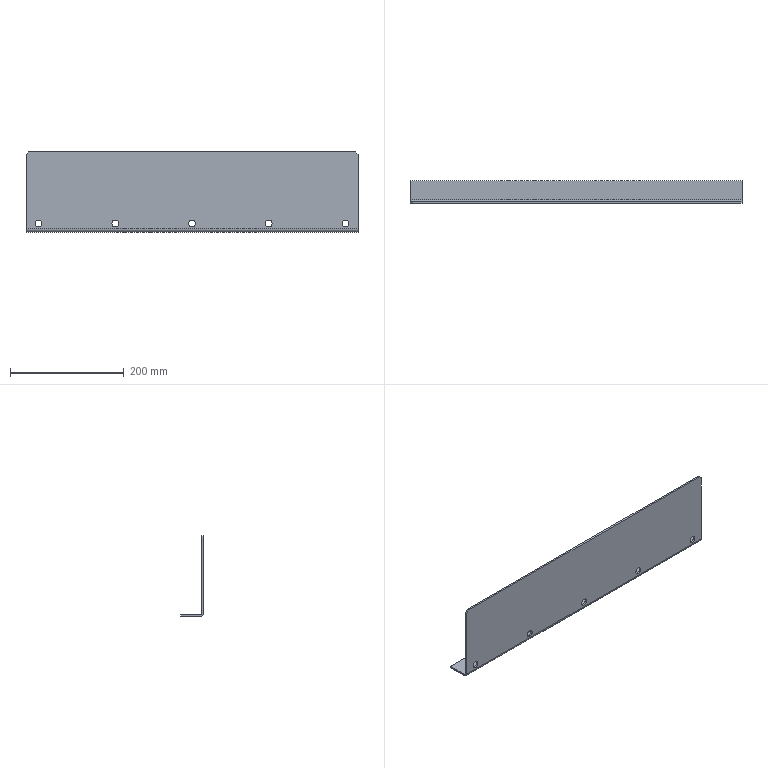Part | STEP file | Produce dryer cooling section-HY-40-M-602 | 1 solid | 26 faces | box 584 x 40 x 142 mm | volume 308453 mm3 | plane 14 | cylinder 12 | commonest cylinder face diameters 12 x11 6 x1
STEP:
#1=CARTESIAN_POINT('',(270.,0.,-120.5));
#2=VERTEX_POINT('',#1);
#3=CARTESIAN_POINT('',(270.,0.,-132.5));
#4=VERTEX_POINT('',#3);
#5=CARTESIAN_POINT('',(270.,0.,-126.5));
#6=DIRECTION('',(0.,-1.,0.));
#7=DIRECTION('',(0.,0.,-1.));
#8=AXIS2_PLACEMENT_3D('',#5,#6,#7);
#9=CIRCLE('',#8,6.);
#10=EDGE_CURVE('',#2,#4,#9,.T.);
#11=ORIENTED_EDGE('',*,*,#10,.T.);
#12=CARTESIAN_POINT('',(270.,3.,-132.5));
#13=VERTEX_POINT('',#12);
#14=CARTESIAN_POINT('',(270.,-7.,-132.5));
#15=DIRECTION('',(0.,1.,0.));
#16=VECTOR('',#15,1000.);
#17=LINE('',#14,#16);
#18=EDGE_CURVE('',#4,#13,#17,.T.);
#19=ORIENTED_EDGE('',*,*,#18,.T.);
#20=CARTESIAN_POINT('',(270.,3.,-120.5));
#21=VERTEX_POINT('',#20);
#22=CARTESIAN_POINT('',(270.,3.,-126.5));
#23=DIRECTION('',(0.,1.,0.));
#24=DIRECTION('',(0.,0.,1.));
#25=AXIS2_PLACEMENT_3D('',#22,#23,#24);
#26=CIRCLE('',#25,6.);
#27=EDGE_CURVE('',#13,#21,#26,.T.);
#28=ORIENTED_EDGE('',*,*,#27,.T.);
#29=CARTESIAN_POINT('',(270.,-7.,-120.5));
#30=DIRECTION('',(0.,1.,0.));
#31=VECTOR('',#30,1000.);
#32=LINE('',#29,#31);
#33=EDGE_CURVE('',#2,#21,#32,.T.);
#34=ORIENTED_EDGE('',*,*,#33,.F.);
#35=EDGE_LOOP('',(#11,#19,#28,#34));
#36=FACE_OUTER_BOUND('',#35,.T.);
#37=CARTESIAN_POINT('',(270.,-7.,-126.5));
#38=DIRECTION('',(0.,1.,0.));
#39=DIRECTION('',(0.,0.,1.));
#40=AXIS2_PLACEMENT_3D('',#37,#38,#39);
#41=CYLINDRICAL_SURFACE('',#40,6.);
#42=ADVANCED_FACE('',(#36),#41,.F.);
#43=CARTESIAN_POINT('',(-135.,0.,-120.5));
#44=VERTEX_POINT('',#43);
#45=CARTESIAN_POINT('',(-135.,0.,-132.5));
#46=VERTEX_POINT('',#45);
#47=CARTESIAN_POINT('',(-135.,0.,-126.5));
#48=DIRECTION('',(0.,-1.,0.));
#49=DIRECTION('',(0.,0.,-1.));
#50=AXIS2_PLACEMENT_3D('',#47,#48,#49);
#51=CIRCLE('',#50,6.);
#52=EDGE_CURVE('',#44,#46,#51,.T.);
#53=ORIENTED_EDGE('',*,*,#52,.T.);
#54=CARTESIAN_POINT('',(-135.,3.,-132.5));
#55=VERTEX_POINT('',#54);
#56=CARTESIAN_POINT('',(-135.,-7.,-132.5));
#57=DIRECTION('',(0.,1.,0.));
#58=VECTOR('',#57,1000.);
#59=LINE('',#56,#58);
#60=EDGE_CURVE('',#46,#55,#59,.T.);
#61=ORIENTED_EDGE('',*,*,#60,.T.);
#62=CARTESIAN_POINT('',(-135.,3.,-120.5));
#63=VERTEX_POINT('',#62);
#64=CARTESIAN_POINT('',(-135.,3.,-126.5));
#65=DIRECTION('',(0.,1.,0.));
#66=DIRECTION('',(0.,0.,1.));
#67=AXIS2_PLACEMENT_3D('',#64,#65,#66);
#68=CIRCLE('',#67,6.);
#69=EDGE_CURVE('',#55,#63,#68,.T.);
#70=ORIENTED_EDGE('',*,*,#69,.T.);
#71=CARTESIAN_POINT('',(-135.,-7.,-120.5));
#72=DIRECTION('',(0.,1.,0.));
#73=VECTOR('',#72,1000.);
#74=LINE('',#71,#73);
#75=EDGE_CURVE('',#44,#63,#74,.T.);
#76=ORIENTED_EDGE('',*,*,#75,.F.);
#77=EDGE_LOOP('',(#53,#61,#70,#76));
#78=FACE_OUTER_BOUND('',#77,.T.);
#79=CARTESIAN_POINT('',(-135.,-7.,-126.5));
#80=DIRECTION('',(0.,1.,0.));
#81=DIRECTION('',(0.,0.,1.));
#82=AXIS2_PLACEMENT_3D('',#79,#80,#81);
#83=CYLINDRICAL_SURFACE('',#82,6.);
#84=ADVANCED_FACE('',(#78),#83,.F.);
#85=CARTESIAN_POINT('',(135.,0.,-120.5));
#86=VERTEX_POINT('',#85);
#87=CARTESIAN_POINT('',(135.,0.,-132.5));
#88=VERTEX_POINT('',#87);
#89=CARTESIAN_POINT('',(135.,0.,-126.5));
#90=DIRECTION('',(0.,-1.,0.));
#91=DIRECTION('',(0.,0.,-1.));
#92=AXIS2_PLACEMENT_3D('',#89,#90,#91);
#93=CIRCLE('',#92,6.);
#94=EDGE_CURVE('',#86,#88,#93,.T.);
#95=ORIENTED_EDGE('',*,*,#94,.T.);
#96=CARTESIAN_POINT('',(135.,3.,-132.5));
#97=VERTEX_POINT('',#96);
#98=CARTESIAN_POINT('',(135.,-7.,-132.5));
#99=DIRECTION('',(0.,1.,0.));
#100=VECTOR('',#99,1000.);
#101=LINE('',#98,#100);
#102=EDGE_CURVE('',#88,#97,#101,.T.);
#103=ORIENTED_EDGE('',*,*,#102,.T.);
#104=CARTESIAN_POINT('',(135.,3.,-120.5));
#105=VERTEX_POINT('',#104);
#106=CARTESIAN_POINT('',(135.,3.,-126.5));
#107=DIRECTION('',(0.,1.,0.));
#108=DIRECTION('',(0.,0.,1.));
#109=AXIS2_PLACEMENT_3D('',#106,#107,#108);
#110=CIRCLE('',#109,6.);
#111=EDGE_CURVE('',#97,#105,#110,.T.);
#112=ORIENTED_EDGE('',*,*,#111,.T.);
#113=CARTESIAN_POINT('',(135.,-7.,-120.5));
#114=DIRECTION('',(0.,1.,0.));
#115=VECTOR('',#114,1000.);
#116=LINE('',#113,#115);
#117=EDGE_CURVE('',#86,#105,#116,.T.);
#118=ORIENTED_EDGE('',*,*,#117,.F.);
#119=EDGE_LOOP('',(#95,#103,#112,#118));
#120=FACE_OUTER_BOUND('',#119,.T.);
#121=CARTESIAN_POINT('',(135.,-7.,-126.5));
#122=DIRECTION('',(0.,1.,0.));
#123=DIRECTION('',(0.,0.,1.));
#124=AXIS2_PLACEMENT_3D('',#121,#122,#123);
#125=CYLINDRICAL_SURFACE('',#124,6.);
#126=ADVANCED_FACE('',(#120),#125,.F.);
#127=CARTESIAN_POINT('',(-270.,0.,-120.5));
#128=VERTEX_POINT('',#127);
#129=CARTESIAN_POINT('',(-270.,0.,-132.5));
#130=VERTEX_POINT('',#129);
#131=CARTESIAN_POINT('',(-270.,0.,-126.5));
#132=DIRECTION('',(0.,-1.,0.));
#133=DIRECTION('',(0.,0.,-1.));
#134=AXIS2_PLACEMENT_3D('',#131,#132,#133);
#135=CIRCLE('',#134,6.);
#136=EDGE_CURVE('',#128,#130,#135,.T.);
#137=ORIENTED_EDGE('',*,*,#136,.T.);
#138=CARTESIAN_POINT('',(-270.,3.,-132.5));
#139=VERTEX_POINT('',#138);
#140=CARTESIAN_POINT('',(-270.,-7.,-132.5));
#141=DIRECTION('',(0.,1.,0.));
#142=VECTOR('',#141,1000.);
#143=LINE('',#140,#142);
#144=EDGE_CURVE('',#130,#139,#143,.T.);
#145=ORIENTED_EDGE('',*,*,#144,.T.);
#146=CARTESIAN_POINT('',(-270.,3.,-120.5));
#147=VERTEX_POINT('',#146);
#148=CARTESIAN_POINT('',(-270.,3.,-126.5));
#149=DIRECTION('',(0.,1.,0.));
#150=DIRECTION('',(0.,0.,1.));
#151=AXIS2_PLACEMENT_3D('',#148,#149,#150);
#152=CIRCLE('',#151,6.);
#153=EDGE_CURVE('',#139,#147,#152,.T.);
#154=ORIENTED_EDGE('',*,*,#153,.T.);
#155=CARTESIAN_POINT('',(-270.,-7.,-120.5));
#156=DIRECTION('',(0.,1.,0.));
#157=VECTOR('',#156,1000.);
#158=LINE('',#155,#157);
#159=EDGE_CURVE('',#128,#147,#158,.T.);
#160=ORIENTED_EDGE('',*,*,#159,.F.);
#161=EDGE_LOOP('',(#137,#145,#154,#160));
#162=FACE_OUTER_BOUND('',#161,.T.);
#163=CARTESIAN_POINT('',(-270.,-7.,-126.5));
#164=DIRECTION('',(0.,1.,0.));
#165=DIRECTION('',(0.,0.,1.));
#166=AXIS2_PLACEMENT_3D('',#163,#164,#165);
#167=CYLINDRICAL_SURFACE('',#166,6.);
#168=ADVANCED_FACE('',(#162),#167,.F.);
#169=CARTESIAN_POINT('',(0.,0.,-120.5));
#170=VERTEX_POINT('',#169);
#171=CARTESIAN_POINT('',(0.,0.,-132.5));
#172=VERTEX_POINT('',#171);
#173=CARTESIAN_POINT('',(0.,0.,-126.5));
#174=DIRECTION('',(0.,-1.,0.));
#175=DIRECTION('',(0.,0.,-1.));
#176=AXIS2_PLACEMENT_3D('',#173,#174,#175);
#177=CIRCLE('',#176,6.);
#178=EDGE_CURVE('',#170,#172,#177,.T.);
#179=ORIENTED_EDGE('',*,*,#178,.T.);
#180=CARTESIAN_POINT('',(0.,3.,-132.5));
#181=VERTEX_POINT('',#180);
#182=CARTESIAN_POINT('',(0.,-7.,-132.5));
#183=DIRECTION('',(0.,1.,0.));
#184=VECTOR('',#183,1000.);
#185=LINE('',#182,#184);
#186=EDGE_CURVE('',#172,#181,#185,.T.);
#187=ORIENTED_EDGE('',*,*,#186,.T.);
#188=CARTESIAN_POINT('',(0.,3.,-120.5));
#189=VERTEX_POINT('',#188);
#190=CARTESIAN_POINT('',(0.,3.,-126.5));
#191=DIRECTION('',(0.,1.,0.));
#192=DIRECTION('',(0.,0.,1.));
#193=AXIS2_PLACEMENT_3D('',#190,#191,#192);
#194=CIRCLE('',#193,6.);
#195=EDGE_CURVE('',#181,#189,#194,.T.);
#196=ORIENTED_EDGE('',*,*,#195,.T.);
#197=CARTESIAN_POINT('',(0.,-7.,-120.5));
#198=DIRECTION('',(0.,1.,0.));
#199=VECTOR('',#198,1000.);
#200=LINE('',#197,#199);
#201=EDGE_CURVE('',#170,#189,#200,.T.);
#202=ORIENTED_EDGE('',*,*,#201,.F.);
#203=EDGE_LOOP('',(#179,#187,#196,#202));
#204=FACE_OUTER_BOUND('',#203,.T.);
#205=CARTESIAN_POINT('',(0.,-7.,-126.5));
#206=DIRECTION('',(0.,1.,0.));
#207=DIRECTION('',(0.,0.,1.));
#208=AXIS2_PLACEMENT_3D('',#205,#206,#207);
#209=CYLINDRICAL_SURFACE('',#208,6.);
#210=ADVANCED_FACE('',(#204),#209,.F.);
#211=CARTESIAN_POINT('',(292.,0.,-136.));
#212=VERTEX_POINT('',#211);
#213=CARTESIAN_POINT('',(292.,3.,-136.));
#214=VERTEX_POINT('',#213);
#215=CARTESIAN_POINT('',(292.,0.,-136.));
#216=DIRECTION('',(0.,1.,0.));
#217=VECTOR('',#216,1000.);
#218=LINE('',#215,#217);
#219=EDGE_CURVE('',#212,#214,#218,.T.);
#220=ORIENTED_EDGE('',*,*,#219,.F.);
#221=CARTESIAN_POINT('',(292.,6.,-142.));
#222=VERTEX_POINT('',#221);
#223=CARTESIAN_POINT('',(292.,6.,-136.));
#224=DIRECTION('',(-1.,0.,0.));
#225=DIRECTION('',(0.,0.,1.));
#226=AXIS2_PLACEMENT_3D('',#223,#224,#225);
#227=CIRCLE('',#226,6.);
#228=EDGE_CURVE('',#222,#212,#227,.T.);
#229=ORIENTED_EDGE('',*,*,#228,.F.);
#230=CARTESIAN_POINT('',(292.,6.,-139.));
#231=VERTEX_POINT('',#230);
#232=CARTESIAN_POINT('',(292.,6.,-139.));
#233=DIRECTION('',(0.,0.,-1.));
#234=VECTOR('',#233,1000.);
#235=LINE('',#232,#234);
#236=EDGE_CURVE('',#231,#222,#235,.T.);
#237=ORIENTED_EDGE('',*,*,#236,.F.);
#238=CARTESIAN_POINT('',(292.,6.,-136.));
#239=DIRECTION('',(-1.,0.,0.));
#240=DIRECTION('',(0.,0.,-1.));
#241=AXIS2_PLACEMENT_3D('',#238,#239,#240);
#242=CIRCLE('',#241,3.);
#243=EDGE_CURVE('',#231,#214,#242,.T.);
#244=ORIENTED_EDGE('',*,*,#243,.T.);
#245=EDGE_LOOP('',(#220,#229,#237,#244));
#246=FACE_OUTER_BOUND('',#245,.T.);
#247=CARTESIAN_POINT('',(292.,0.,-136.));
#248=DIRECTION('',(1.,0.,0.));
#249=DIRECTION('',(0.,0.,-1.));
#250=AXIS2_PLACEMENT_3D('',#247,#248,#249);
#251=PLANE('',#250);
#252=ADVANCED_FACE('',(#246),#251,.T.);
#253=CARTESIAN_POINT('',(292.,3.,-5.));
#254=VERTEX_POINT('',#253);
#255=CARTESIAN_POINT('',(292.,3.,0.));
#256=DIRECTION('',(0.,0.,1.));
#257=VECTOR('',#256,1000.);
#258=LINE('',#255,#257);
#259=EDGE_CURVE('',#214,#254,#258,.T.);
#260=ORIENTED_EDGE('',*,*,#259,.T.);
#261=CARTESIAN_POINT('',(292.,0.,-5.));
#262=VERTEX_POINT('',#261);
#263=CARTESIAN_POINT('',(292.,6.,-5.));
#264=DIRECTION('',(0.,-1.,0.));
#265=VECTOR('',#264,1000.);
#266=LINE('',#263,#265);
#267=EDGE_CURVE('',#254,#262,#266,.T.);
#268=ORIENTED_EDGE('',*,*,#267,.T.);
#269=CARTESIAN_POINT('',(292.,0.,0.));
#270=DIRECTION('',(0.,0.,1.));
#271=VECTOR('',#270,1000.);
#272=LINE('',#269,#271);
#273=EDGE_CURVE('',#212,#262,#272,.T.);
#274=ORIENTED_EDGE('',*,*,#273,.F.);
#275=ORIENTED_EDGE('',*,*,#219,.T.);
#276=EDGE_LOOP('',(#260,#268,#274,#275));
#277=FACE_OUTER_BOUND('',#276,.T.);
#278=CARTESIAN_POINT('',(292.,6.,-139.));
#279=DIRECTION('',(1.,0.,0.));
#280=DIRECTION('',(0.,0.,-1.));
#281=AXIS2_PLACEMENT_3D('',#278,#279,#280);
#282=PLANE('',#281);
#283=ADVANCED_FACE('',(#277),#282,.T.);
#284=CARTESIAN_POINT('',(-292.,6.,-142.));
#285=VERTEX_POINT('',#284);
#286=CARTESIAN_POINT('',(-292.,6.,-139.));
#287=VERTEX_POINT('',#286);
#288=CARTESIAN_POINT('',(-292.,6.,-142.));
#289=DIRECTION('',(0.,0.,1.));
#290=VECTOR('',#289,1000.);
#291=LINE('',#288,#290);
#292=EDGE_CURVE('',#285,#287,#291,.T.);
#293=ORIENTED_EDGE('',*,*,#292,.F.);
#294=CARTESIAN_POINT('',(-292.,0.,-136.));
#295=VERTEX_POINT('',#294);
#296=CARTESIAN_POINT('',(-292.,6.,-136.));
#297=DIRECTION('',(-1.,0.,0.));
#298=DIRECTION('',(0.,0.,1.));
#299=AXIS2_PLACEMENT_3D('',#296,#297,#298);
#300=CIRCLE('',#299,6.);
#301=EDGE_CURVE('',#285,#295,#300,.T.);
#302=ORIENTED_EDGE('',*,*,#301,.T.);
#303=CARTESIAN_POINT('',(-292.,3.,-136.));
#304=VERTEX_POINT('',#303);
#305=CARTESIAN_POINT('',(-292.,3.,-136.));
#306=DIRECTION('',(0.,-1.,0.));
#307=VECTOR('',#306,1000.);
#308=LINE('',#305,#307);
#309=EDGE_CURVE('',#304,#295,#308,.T.);
#310=ORIENTED_EDGE('',*,*,#309,.F.);
#311=CARTESIAN_POINT('',(-292.,6.,-136.));
#312=DIRECTION('',(-1.,0.,0.));
#313=DIRECTION('',(0.,0.,-1.));
#314=AXIS2_PLACEMENT_3D('',#311,#312,#313);
#315=CIRCLE('',#314,3.);
#316=EDGE_CURVE('',#287,#304,#315,.T.);
#317=ORIENTED_EDGE('',*,*,#316,.F.);
#318=EDGE_LOOP('',(#293,#302,#310,#317));
#319=FACE_OUTER_BOUND('',#318,.T.);
#320=CARTESIAN_POINT('',(-292.,6.,-142.));
#321=DIRECTION('',(-1.,0.,0.));
#322=DIRECTION('',(0.,0.,1.));
#323=AXIS2_PLACEMENT_3D('',#320,#321,#322);
#324=PLANE('',#323);
#325=ADVANCED_FACE('',(#319),#324,.T.);
#326=CARTESIAN_POINT('',(-292.,40.,-142.));
#327=VERTEX_POINT('',#326);
#328=CARTESIAN_POINT('',(-292.,0.,-142.));
#329=DIRECTION('',(0.,-1.,0.));
#330=VECTOR('',#329,1000.);
#331=LINE('',#328,#330);
#332=EDGE_CURVE('',#327,#285,#331,.T.);
#333=ORIENTED_EDGE('',*,*,#332,.T.);
#334=ORIENTED_EDGE('',*,*,#292,.T.);
#335=CARTESIAN_POINT('',(-292.,40.,-139.));
#336=VERTEX_POINT('',#335);
#337=CARTESIAN_POINT('',(-292.,0.,-139.));
#338=DIRECTION('',(0.,-1.,0.));
#339=VECTOR('',#338,1000.);
#340=LINE('',#337,#339);
#341=EDGE_CURVE('',#336,#287,#340,.T.);
#342=ORIENTED_EDGE('',*,*,#341,.F.);
#343=CARTESIAN_POINT('',(-292.,40.,-139.));
#344=DIRECTION('',(0.,0.,-1.));
#345=VECTOR('',#344,1000.);
#346=LINE('',#343,#345);
#347=EDGE_CURVE('',#336,#327,#346,.T.);
#348=ORIENTED_EDGE('',*,*,#347,.T.);
#349=EDGE_LOOP('',(#333,#334,#342,#348));
#350=FACE_OUTER_BOUND('',#349,.T.);
#351=CARTESIAN_POINT('',(-292.,3.,-136.));
#352=DIRECTION('',(-1.,0.,0.));
#353=DIRECTION('',(0.,0.,1.));
#354=AXIS2_PLACEMENT_3D('',#351,#352,#353);
#355=PLANE('',#354);
#356=ADVANCED_FACE('',(#350),#355,.T.);
#357=CARTESIAN_POINT('',(270.,3.,-126.5));
#358=DIRECTION('',(0.,1.,0.));
#359=DIRECTION('',(0.,0.,1.));
#360=AXIS2_PLACEMENT_3D('',#357,#358,#359);
#361=CIRCLE('',#360,6.);
#362=EDGE_CURVE('',#21,#13,#361,.T.);
#363=ORIENTED_EDGE('',*,*,#362,.F.);
#364=ORIENTED_EDGE('',*,*,#27,.F.);
#365=EDGE_LOOP('',(#363,#364));
#366=FACE_BOUND('',#365,.T.);
#367=CARTESIAN_POINT('',(-135.,3.,-126.5));
#368=DIRECTION('',(0.,1.,0.));
#369=DIRECTION('',(0.,0.,1.));
#370=AXIS2_PLACEMENT_3D('',#367,#368,#369);
#371=CIRCLE('',#370,6.);
#372=EDGE_CURVE('',#63,#55,#371,.T.);
#373=ORIENTED_EDGE('',*,*,#372,.F.);
#374=ORIENTED_EDGE('',*,*,#69,.F.);
#375=EDGE_LOOP('',(#373,#374));
#376=FACE_BOUND('',#375,.T.);
#377=CARTESIAN_POINT('',(135.,3.,-126.5));
#378=DIRECTION('',(0.,1.,0.));
#379=DIRECTION('',(0.,0.,1.));
#380=AXIS2_PLACEMENT_3D('',#377,#378,#379);
#381=CIRCLE('',#380,6.);
#382=EDGE_CURVE('',#105,#97,#381,.T.);
#383=ORIENTED_EDGE('',*,*,#382,.F.);
#384=ORIENTED_EDGE('',*,*,#111,.F.);
#385=EDGE_LOOP('',(#383,#384));
#386=FACE_BOUND('',#385,.T.);
#387=CARTESIAN_POINT('',(-270.,3.,-126.5));
#388=DIRECTION('',(0.,1.,0.));
#389=DIRECTION('',(0.,0.,1.));
#390=AXIS2_PLACEMENT_3D('',#387,#388,#389);
#391=CIRCLE('',#390,6.);
#392=EDGE_CURVE('',#147,#139,#391,.T.);
#393=ORIENTED_EDGE('',*,*,#392,.F.);
#394=ORIENTED_EDGE('',*,*,#153,.F.);
#395=EDGE_LOOP('',(#393,#394));
#396=FACE_BOUND('',#395,.T.);
#397=CARTESIAN_POINT('',(0.,3.,-126.5));
#398=DIRECTION('',(0.,1.,0.));
#399=DIRECTION('',(0.,0.,1.));
#400=AXIS2_PLACEMENT_3D('',#397,#398,#399);
#401=CIRCLE('',#400,6.);
#402=EDGE_CURVE('',#189,#181,#401,.T.);
#403=ORIENTED_EDGE('',*,*,#402,.F.);
#404=ORIENTED_EDGE('',*,*,#195,.F.);
#405=EDGE_LOOP('',(#403,#404));
#406=FACE_BOUND('',#405,.T.);
#407=CARTESIAN_POINT('',(-292.,3.,-5.));
#408=VERTEX_POINT('',#407);
#409=CARTESIAN_POINT('',(-292.,3.,0.));
#410=DIRECTION('',(0.,0.,1.));
#411=VECTOR('',#410,1000.);
#412=LINE('',#409,#411);
#413=EDGE_CURVE('',#304,#408,#412,.T.);
#414=ORIENTED_EDGE('',*,*,#413,.T.);
#415=CARTESIAN_POINT('',(-287.,3.,0.));
#416=VERTEX_POINT('',#415);
#417=CARTESIAN_POINT('',(-292.,3.,-5.));
#418=DIRECTION('',(0.7071,0.,0.7071));
#419=VECTOR('',#418,1000.);
#420=LINE('',#417,#419);
#421=EDGE_CURVE('',#408,#416,#420,.T.);
#422=ORIENTED_EDGE('',*,*,#421,.T.);
#423=CARTESIAN_POINT('',(287.,3.,0.));
#424=VERTEX_POINT('',#423);
#425=CARTESIAN_POINT('',(292.,3.,0.));
#426=DIRECTION('',(-1.,0.,0.));
#427=VECTOR('',#426,1000.);
#428=LINE('',#425,#427);
#429=EDGE_CURVE('',#424,#416,#428,.T.);
#430=ORIENTED_EDGE('',*,*,#429,.F.);
#431=CARTESIAN_POINT('',(287.,3.,0.));
#432=DIRECTION('',(0.7071,0.,-0.7071));
#433=VECTOR('',#432,1000.);
#434=LINE('',#431,#433);
#435=EDGE_CURVE('',#424,#254,#434,.T.);
#436=ORIENTED_EDGE('',*,*,#435,.T.);
#437=ORIENTED_EDGE('',*,*,#259,.F.);
#438=CARTESIAN_POINT('',(292.,3.,-136.));
#439=DIRECTION('',(-1.,0.,0.));
#440=VECTOR('',#439,1000.);
#441=LINE('',#438,#440);
#442=EDGE_CURVE('',#214,#304,#441,.T.);
#443=ORIENTED_EDGE('',*,*,#442,.T.);
#444=EDGE_LOOP('',(#414,#422,#430,#436,#437,#443));
#445=FACE_OUTER_BOUND('',#444,.T.);
#446=CARTESIAN_POINT('',(292.,3.,0.));
#447=DIRECTION('',(0.,-1.,0.));
#448=DIRECTION('',(0.,0.,-1.));
#449=AXIS2_PLACEMENT_3D('',#446,#447,#448);
#450=PLANE('',#449);
#451=ADVANCED_FACE('',(#366,#376,#386,#396,#406,#445),#450,.F.);
#452=ORIENTED_EDGE('',*,*,#429,.T.);
#453=CARTESIAN_POINT('',(-287.,0.,0.));
#454=VERTEX_POINT('',#453);
#455=CARTESIAN_POINT('',(-287.,0.,0.));
#456=DIRECTION('',(0.,-1.,0.));
#457=VECTOR('',#456,1000.);
#458=LINE('',#455,#457);
#459=EDGE_CURVE('',#416,#454,#458,.T.);
#460=ORIENTED_EDGE('',*,*,#459,.T.);
#461=CARTESIAN_POINT('',(287.,0.,0.));
#462=VERTEX_POINT('',#461);
#463=CARTESIAN_POINT('',(292.,0.,0.));
#464=DIRECTION('',(-1.,0.,0.));
#465=VECTOR('',#464,1000.);
#466=LINE('',#463,#465);
#467=EDGE_CURVE('',#462,#454,#466,.T.);
#468=ORIENTED_EDGE('',*,*,#467,.F.);
#469=CARTESIAN_POINT('',(287.,0.,0.));
#470=DIRECTION('',(0.,1.,0.));
#471=VECTOR('',#470,1000.);
#472=LINE('',#469,#471);
#473=EDGE_CURVE('',#462,#424,#472,.T.);
#474=ORIENTED_EDGE('',*,*,#473,.T.);
#475=EDGE_LOOP('',(#452,#460,#468,#474));
#476=FACE_OUTER_BOUND('',#475,.T.);
#477=CARTESIAN_POINT('',(292.,0.,0.));
#478=DIRECTION('',(0.,0.,1.));
#479=DIRECTION('',(1.,0.,0.));
#480=AXIS2_PLACEMENT_3D('',#477,#478,#479);
#481=PLANE('',#480);
#482=ADVANCED_FACE('',(#476),#481,.T.);
#483=ORIENTED_EDGE('',*,*,#10,.F.);
#484=CARTESIAN_POINT('',(270.,0.,-126.5));
#485=DIRECTION('',(0.,-1.,0.));
#486=DIRECTION('',(0.,0.,-1.));
#487=AXIS2_PLACEMENT_3D('',#484,#485,#486);
#488=CIRCLE('',#487,6.);
#489=EDGE_CURVE('',#4,#2,#488,.T.);
#490=ORIENTED_EDGE('',*,*,#489,.F.);
#491=EDGE_LOOP('',(#483,#490));
#492=FACE_BOUND('',#491,.T.);
#493=ORIENTED_EDGE('',*,*,#52,.F.);
#494=CARTESIAN_POINT('',(-135.,0.,-126.5));
#495=DIRECTION('',(0.,-1.,0.));
#496=DIRECTION('',(0.,0.,-1.));
#497=AXIS2_PLACEMENT_3D('',#494,#495,#496);
#498=CIRCLE('',#497,6.);
#499=EDGE_CURVE('',#46,#44,#498,.T.);
#500=ORIENTED_EDGE('',*,*,#499,.F.);
#501=EDGE_LOOP('',(#493,#500));
#502=FACE_BOUND('',#501,.T.);
#503=ORIENTED_EDGE('',*,*,#94,.F.);
#504=CARTESIAN_POINT('',(135.,0.,-126.5));
#505=DIRECTION('',(0.,-1.,0.));
#506=DIRECTION('',(0.,0.,-1.));
#507=AXIS2_PLACEMENT_3D('',#504,#505,#506);
#508=CIRCLE('',#507,6.);
#509=EDGE_CURVE('',#88,#86,#508,.T.);
#510=ORIENTED_EDGE('',*,*,#509,.F.);
#511=EDGE_LOOP('',(#503,#510));
#512=FACE_BOUND('',#511,.T.);
#513=ORIENTED_EDGE('',*,*,#136,.F.);
#514=CARTESIAN_POINT('',(-270.,0.,-126.5));
#515=DIRECTION('',(0.,-1.,0.));
#516=DIRECTION('',(0.,0.,-1.));
#517=AXIS2_PLACEMENT_3D('',#514,#515,#516);
#518=CIRCLE('',#517,6.);
#519=EDGE_CURVE('',#130,#128,#518,.T.);
#520=ORIENTED_EDGE('',*,*,#519,.F.);
#521=EDGE_LOOP('',(#513,#520));
#522=FACE_BOUND('',#521,.T.);
#523=ORIENTED_EDGE('',*,*,#178,.F.);
#524=CARTESIAN_POINT('',(0.,0.,-126.5));
#525=DIRECTION('',(0.,-1.,0.));
#526=DIRECTION('',(0.,0.,-1.));
#527=AXIS2_PLACEMENT_3D('',#524,#525,#526);
#528=CIRCLE('',#527,6.);
#529=EDGE_CURVE('',#172,#170,#528,.T.);
#530=ORIENTED_EDGE('',*,*,#529,.F.);
#531=EDGE_LOOP('',(#523,#530));
#532=FACE_BOUND('',#531,.T.);
#533=ORIENTED_EDGE('',*,*,#467,.T.);
#534=CARTESIAN_POINT('',(-292.,0.,-5.));
#535=VERTEX_POINT('',#534);
#536=CARTESIAN_POINT('',(2.5,0.,289.5));
#537=DIRECTION('',(-0.7071,0.,-0.7071));
#538=VECTOR('',#537,1000.);
#539=LINE('',#536,#538);
#540=EDGE_CURVE('',#454,#535,#539,.T.);
#541=ORIENTED_EDGE('',*,*,#540,.T.);
#542=CARTESIAN_POINT('',(-292.,0.,0.));
#543=DIRECTION('',(0.,0.,1.));
#544=VECTOR('',#543,1000.);
#545=LINE('',#542,#544);
#546=EDGE_CURVE('',#295,#535,#545,.T.);
#547=ORIENTED_EDGE('',*,*,#546,.F.);
#548=CARTESIAN_POINT('',(292.,0.,-136.));
#549=DIRECTION('',(-1.,0.,0.));
#550=VECTOR('',#549,1000.);
#551=LINE('',#548,#550);
#552=EDGE_CURVE('',#212,#295,#551,.T.);
#553=ORIENTED_EDGE('',*,*,#552,.F.);
#554=ORIENTED_EDGE('',*,*,#273,.T.);
#555=CARTESIAN_POINT('',(289.5,0.,-2.5));
#556=DIRECTION('',(-0.7071,0.,0.7071));
#557=VECTOR('',#556,1000.);
#558=LINE('',#555,#557);
#559=EDGE_CURVE('',#262,#462,#558,.T.);
#560=ORIENTED_EDGE('',*,*,#559,.T.);
#561=EDGE_LOOP('',(#533,#541,#547,#553,#554,#560));
#562=FACE_OUTER_BOUND('',#561,.T.);
#563=CARTESIAN_POINT('',(292.,0.,0.));
#564=DIRECTION('',(0.,-1.,0.));
#565=DIRECTION('',(0.,0.,-1.));
#566=AXIS2_PLACEMENT_3D('',#563,#564,#565);
#567=PLANE('',#566);
#568=ADVANCED_FACE('',(#492,#502,#512,#522,#532,#562),#567,.T.);
#569=ORIENTED_EDGE('',*,*,#301,.F.);
#570=CARTESIAN_POINT('',(292.,6.,-142.));
#571=DIRECTION('',(-1.,0.,0.));
#572=VECTOR('',#571,1000.);
#573=LINE('',#570,#572);
#574=EDGE_CURVE('',#222,#285,#573,.T.);
#575=ORIENTED_EDGE('',*,*,#574,.F.);
#576=ORIENTED_EDGE('',*,*,#228,.T.);
#577=ORIENTED_EDGE('',*,*,#552,.T.);
#578=EDGE_LOOP('',(#569,#575,#576,#577));
#579=FACE_OUTER_BOUND('',#578,.T.);
#580=CARTESIAN_POINT('',(292.,6.,-136.));
#581=DIRECTION('',(-1.,0.,0.));
#582=DIRECTION('',(0.,0.,1.));
#583=AXIS2_PLACEMENT_3D('',#580,#581,#582);
#584=CYLINDRICAL_SURFACE('',#583,6.);
#585=ADVANCED_FACE('',(#579),#584,.T.);
#586=ORIENTED_EDGE('',*,*,#332,.F.);
#587=CARTESIAN_POINT('',(292.,40.,-142.));
#588=VERTEX_POINT('',#587);
#589=CARTESIAN_POINT('',(292.,40.,-142.));
#590=DIRECTION('',(-1.,0.,0.));
#591=VECTOR('',#590,1000.);
#592=LINE('',#589,#591);
#593=EDGE_CURVE('',#588,#327,#592,.T.);
#594=ORIENTED_EDGE('',*,*,#593,.F.);
#595=CARTESIAN_POINT('',(292.,0.,-142.));
#596=DIRECTION('',(0.,-1.,0.));
#597=VECTOR('',#596,1000.);
#598=LINE('',#595,#597);
#599=EDGE_CURVE('',#588,#222,#598,.T.);
#600=ORIENTED_EDGE('',*,*,#599,.T.);
#601=ORIENTED_EDGE('',*,*,#574,.T.);
#602=EDGE_LOOP('',(#586,#594,#600,#601));
#603=FACE_OUTER_BOUND('',#602,.T.);
#604=CARTESIAN_POINT('',(292.,0.,-142.));
#605=DIRECTION('',(0.,0.,-1.));
#606=DIRECTION('',(-1.,0.,0.));
#607=AXIS2_PLACEMENT_3D('',#604,#605,#606);
#608=PLANE('',#607);
#609=ADVANCED_FACE('',(#603),#608,.T.);
#610=ORIENTED_EDGE('',*,*,#347,.F.);
#611=CARTESIAN_POINT('',(292.,40.,-139.));
#612=VERTEX_POINT('',#611);
#613=CARTESIAN_POINT('',(292.,40.,-139.));
#614=DIRECTION('',(-1.,0.,0.));
#615=VECTOR('',#614,1000.);
#616=LINE('',#613,#615);
#617=EDGE_CURVE('',#612,#336,#616,.T.);
#618=ORIENTED_EDGE('',*,*,#617,.F.);
#619=CARTESIAN_POINT('',(292.,40.,-139.));
#620=DIRECTION('',(0.,0.,-1.));
#621=VECTOR('',#620,1000.);
#622=LINE('',#619,#621);
#623=EDGE_CURVE('',#612,#588,#622,.T.);
#624=ORIENTED_EDGE('',*,*,#623,.T.);
#625=ORIENTED_EDGE('',*,*,#593,.T.);
#626=EDGE_LOOP('',(#610,#618,#624,#625));
#627=FACE_OUTER_BOUND('',#626,.T.);
#628=CARTESIAN_POINT('',(292.,40.,-139.));
#629=DIRECTION('',(0.,1.,0.));
#630=DIRECTION('',(0.,0.,1.));
#631=AXIS2_PLACEMENT_3D('',#628,#629,#630);
#632=PLANE('',#631);
#633=ADVANCED_FACE('',(#627),#632,.T.);
#634=ORIENTED_EDGE('',*,*,#341,.T.);
#635=CARTESIAN_POINT('',(292.,6.,-139.));
#636=DIRECTION('',(-1.,0.,0.));
#637=VECTOR('',#636,1000.);
#638=LINE('',#635,#637);
#639=EDGE_CURVE('',#231,#287,#638,.T.);
#640=ORIENTED_EDGE('',*,*,#639,.F.);
#641=CARTESIAN_POINT('',(292.,0.,-139.));
#642=DIRECTION('',(0.,-1.,0.));
#643=VECTOR('',#642,1000.);
#644=LINE('',#641,#643);
#645=EDGE_CURVE('',#612,#231,#644,.T.);
#646=ORIENTED_EDGE('',*,*,#645,.F.);
#647=ORIENTED_EDGE('',*,*,#617,.T.);
#648=EDGE_LOOP('',(#634,#640,#646,#647));
#649=FACE_OUTER_BOUND('',#648,.T.);
#650=CARTESIAN_POINT('',(292.,0.,-139.));
#651=DIRECTION('',(0.,0.,-1.));
#652=DIRECTION('',(-1.,0.,0.));
#653=AXIS2_PLACEMENT_3D('',#650,#651,#652);
#654=PLANE('',#653);
#655=ADVANCED_FACE('',(#649),#654,.F.);
#656=ORIENTED_EDGE('',*,*,#316,.T.);
#657=ORIENTED_EDGE('',*,*,#442,.F.);
#658=ORIENTED_EDGE('',*,*,#243,.F.);
#659=ORIENTED_EDGE('',*,*,#639,.T.);
#660=EDGE_LOOP('',(#656,#657,#658,#659));
#661=FACE_OUTER_BOUND('',#660,.T.);
#662=CARTESIAN_POINT('',(292.,6.,-136.));
#663=DIRECTION('',(-1.,0.,0.));
#664=DIRECTION('',(0.,0.,1.));
#665=AXIS2_PLACEMENT_3D('',#662,#663,#664);
#666=CYLINDRICAL_SURFACE('',#665,3.);
#667=ADVANCED_FACE('',(#661),#666,.F.);
#668=ORIENTED_EDGE('',*,*,#645,.T.);
#669=ORIENTED_EDGE('',*,*,#236,.T.);
#670=ORIENTED_EDGE('',*,*,#599,.F.);
#671=ORIENTED_EDGE('',*,*,#623,.F.);
#672=EDGE_LOOP('',(#668,#669,#670,#671));
#673=FACE_OUTER_BOUND('',#672,.T.);
#674=CARTESIAN_POINT('',(292.,6.,-136.));
#675=DIRECTION('',(-1.,0.,0.));
#676=DIRECTION('',(0.,0.,1.));
#677=AXIS2_PLACEMENT_3D('',#674,#675,#676);
#678=PLANE('',#677);
#679=ADVANCED_FACE('',(#673),#678,.F.);
#680=ORIENTED_EDGE('',*,*,#546,.T.);
#681=CARTESIAN_POINT('',(-292.,6.,-5.));
#682=DIRECTION('',(0.,1.,0.));
#683=VECTOR('',#682,1000.);
#684=LINE('',#681,#683);
#685=EDGE_CURVE('',#535,#408,#684,.T.);
#686=ORIENTED_EDGE('',*,*,#685,.T.);
#687=ORIENTED_EDGE('',*,*,#413,.F.);
#688=ORIENTED_EDGE('',*,*,#309,.T.);
#689=EDGE_LOOP('',(#680,#686,#687,#688));
#690=FACE_OUTER_BOUND('',#689,.T.);
#691=CARTESIAN_POINT('',(-292.,6.,-136.));
#692=DIRECTION('',(-1.,0.,0.));
#693=DIRECTION('',(0.,0.,1.));
#694=AXIS2_PLACEMENT_3D('',#691,#692,#693);
#695=PLANE('',#694);
#696=ADVANCED_FACE('',(#690),#695,.T.);
#697=ORIENTED_EDGE('',*,*,#540,.F.);
#698=ORIENTED_EDGE('',*,*,#459,.F.);
#699=ORIENTED_EDGE('',*,*,#421,.F.);
#700=ORIENTED_EDGE('',*,*,#685,.F.);
#701=EDGE_LOOP('',(#697,#698,#699,#700));
#702=FACE_OUTER_BOUND('',#701,.T.);
#703=CARTESIAN_POINT('',(-292.,6.,-5.));
#704=DIRECTION('',(0.7071,0.,-0.7071));
#705=DIRECTION('',(0.,1.,0.));
#706=AXIS2_PLACEMENT_3D('',#703,#704,#705);
#707=PLANE('',#706);
#708=ADVANCED_FACE('',(#702),#707,.F.);
#709=ORIENTED_EDGE('',*,*,#559,.F.);
#710=ORIENTED_EDGE('',*,*,#267,.F.);
#711=ORIENTED_EDGE('',*,*,#435,.F.);
#712=ORIENTED_EDGE('',*,*,#473,.F.);
#713=EDGE_LOOP('',(#709,#710,#711,#712));
#714=FACE_OUTER_BOUND('',#713,.T.);
#715=CARTESIAN_POINT('',(287.,0.,0.));
#716=DIRECTION('',(-0.7071,0.,-0.7071));
#717=DIRECTION('',(0.,1.,0.));
#718=AXIS2_PLACEMENT_3D('',#715,#716,#717);
#719=PLANE('',#718);
#720=ADVANCED_FACE('',(#714),#719,.F.);
#721=ORIENTED_EDGE('',*,*,#186,.F.);
#722=ORIENTED_EDGE('',*,*,#529,.T.);
#723=ORIENTED_EDGE('',*,*,#201,.T.);
#724=ORIENTED_EDGE('',*,*,#402,.T.);
#725=EDGE_LOOP('',(#721,#722,#723,#724));
#726=FACE_OUTER_BOUND('',#725,.T.);
#727=CARTESIAN_POINT('',(0.,-7.,-126.5));
#728=DIRECTION('',(0.,1.,0.));
#729=DIRECTION('',(0.,0.,1.));
#730=AXIS2_PLACEMENT_3D('',#727,#728,#729);
#731=CYLINDRICAL_SURFACE('',#730,6.);
#732=ADVANCED_FACE('',(#726),#731,.F.);
#733=ORIENTED_EDGE('',*,*,#144,.F.);
#734=ORIENTED_EDGE('',*,*,#519,.T.);
#735=ORIENTED_EDGE('',*,*,#159,.T.);
#736=ORIENTED_EDGE('',*,*,#392,.T.);
#737=EDGE_LOOP('',(#733,#734,#735,#736));
#738=FACE_OUTER_BOUND('',#737,.T.);
#739=CARTESIAN_POINT('',(-270.,-7.,-126.5));
#740=DIRECTION('',(0.,1.,0.));
#741=DIRECTION('',(0.,0.,1.));
#742=AXIS2_PLACEMENT_3D('',#739,#740,#741);
#743=CYLINDRICAL_SURFACE('',#742,6.);
#744=ADVANCED_FACE('',(#738),#743,.F.);
#745=ORIENTED_EDGE('',*,*,#102,.F.);
#746=ORIENTED_EDGE('',*,*,#509,.T.);
#747=ORIENTED_EDGE('',*,*,#117,.T.);
#748=ORIENTED_EDGE('',*,*,#382,.T.);
#749=EDGE_LOOP('',(#745,#746,#747,#748));
#750=FACE_OUTER_BOUND('',#749,.T.);
#751=CARTESIAN_POINT('',(135.,-7.,-126.5));
#752=DIRECTION('',(0.,1.,0.));
#753=DIRECTION('',(0.,0.,1.));
#754=AXIS2_PLACEMENT_3D('',#751,#752,#753);
#755=CYLINDRICAL_SURFACE('',#754,6.);
#756=ADVANCED_FACE('',(#750),#755,.F.);
#757=ORIENTED_EDGE('',*,*,#60,.F.);
#758=ORIENTED_EDGE('',*,*,#499,.T.);
#759=ORIENTED_EDGE('',*,*,#75,.T.);
#760=ORIENTED_EDGE('',*,*,#372,.T.);
#761=EDGE_LOOP('',(#757,#758,#759,#760));
#762=FACE_OUTER_BOUND('',#761,.T.);
#763=CARTESIAN_POINT('',(-135.,-7.,-126.5));
#764=DIRECTION('',(0.,1.,0.));
#765=DIRECTION('',(0.,0.,1.));
#766=AXIS2_PLACEMENT_3D('',#763,#764,#765);
#767=CYLINDRICAL_SURFACE('',#766,6.);
#768=ADVANCED_FACE('',(#762),#767,.F.);
#769=ORIENTED_EDGE('',*,*,#18,.F.);
#770=ORIENTED_EDGE('',*,*,#489,.T.);
#771=ORIENTED_EDGE('',*,*,#33,.T.);
#772=ORIENTED_EDGE('',*,*,#362,.T.);
#773=EDGE_LOOP('',(#769,#770,#771,#772));
#774=FACE_OUTER_BOUND('',#773,.T.);
#775=CARTESIAN_POINT('',(270.,-7.,-126.5));
#776=DIRECTION('',(0.,1.,0.));
#777=DIRECTION('',(0.,0.,1.));
#778=AXIS2_PLACEMENT_3D('',#775,#776,#777);
#779=CYLINDRICAL_SURFACE('',#778,6.);
#780=ADVANCED_FACE('',(#774),#779,.F.);
#781=CLOSED_SHELL('',(#42,#84,#126,#168,#210,#252,#283,#325,#356,#451,#482,#568,#585,#609,#633,#655,#667,#679,#696,#708,#720,#732,#744,#756,#768,#780));
#782=MANIFOLD_SOLID_BREP('',#781);
#783=CARTESIAN_POINT('',(0.,0.,0.));
#784=DIRECTION('',(0.,0.,1.));
#785=DIRECTION('',(1.,0.,0.));
#786=AXIS2_PLACEMENT_3D('',#783,#784,#785);
#787=(LENGTH_UNIT()NAMED_UNIT(*)SI_UNIT(.MILLI.,.METRE.));
#788=UNCERTAINTY_MEASURE_WITH_UNIT(LENGTH_MEASURE(0.00001),#787,'','');
#789=(NAMED_UNIT(*)PLANE_ANGLE_UNIT()SI_UNIT($,.RADIAN.));
#790=(NAMED_UNIT(*)SI_UNIT($,.STERADIAN.)SOLID_ANGLE_UNIT());
#791=(GEOMETRIC_REPRESENTATION_CONTEXT(3)GLOBAL_UNCERTAINTY_ASSIGNED_CONTEXT((#788))GLOBAL_UNIT_ASSIGNED_CONTEXT((#787,#789,#790))REPRESENTATION_CONTEXT('',''));
#792=ADVANCED_BREP_SHAPE_REPRESENTATION('',(#782,#786),#791);